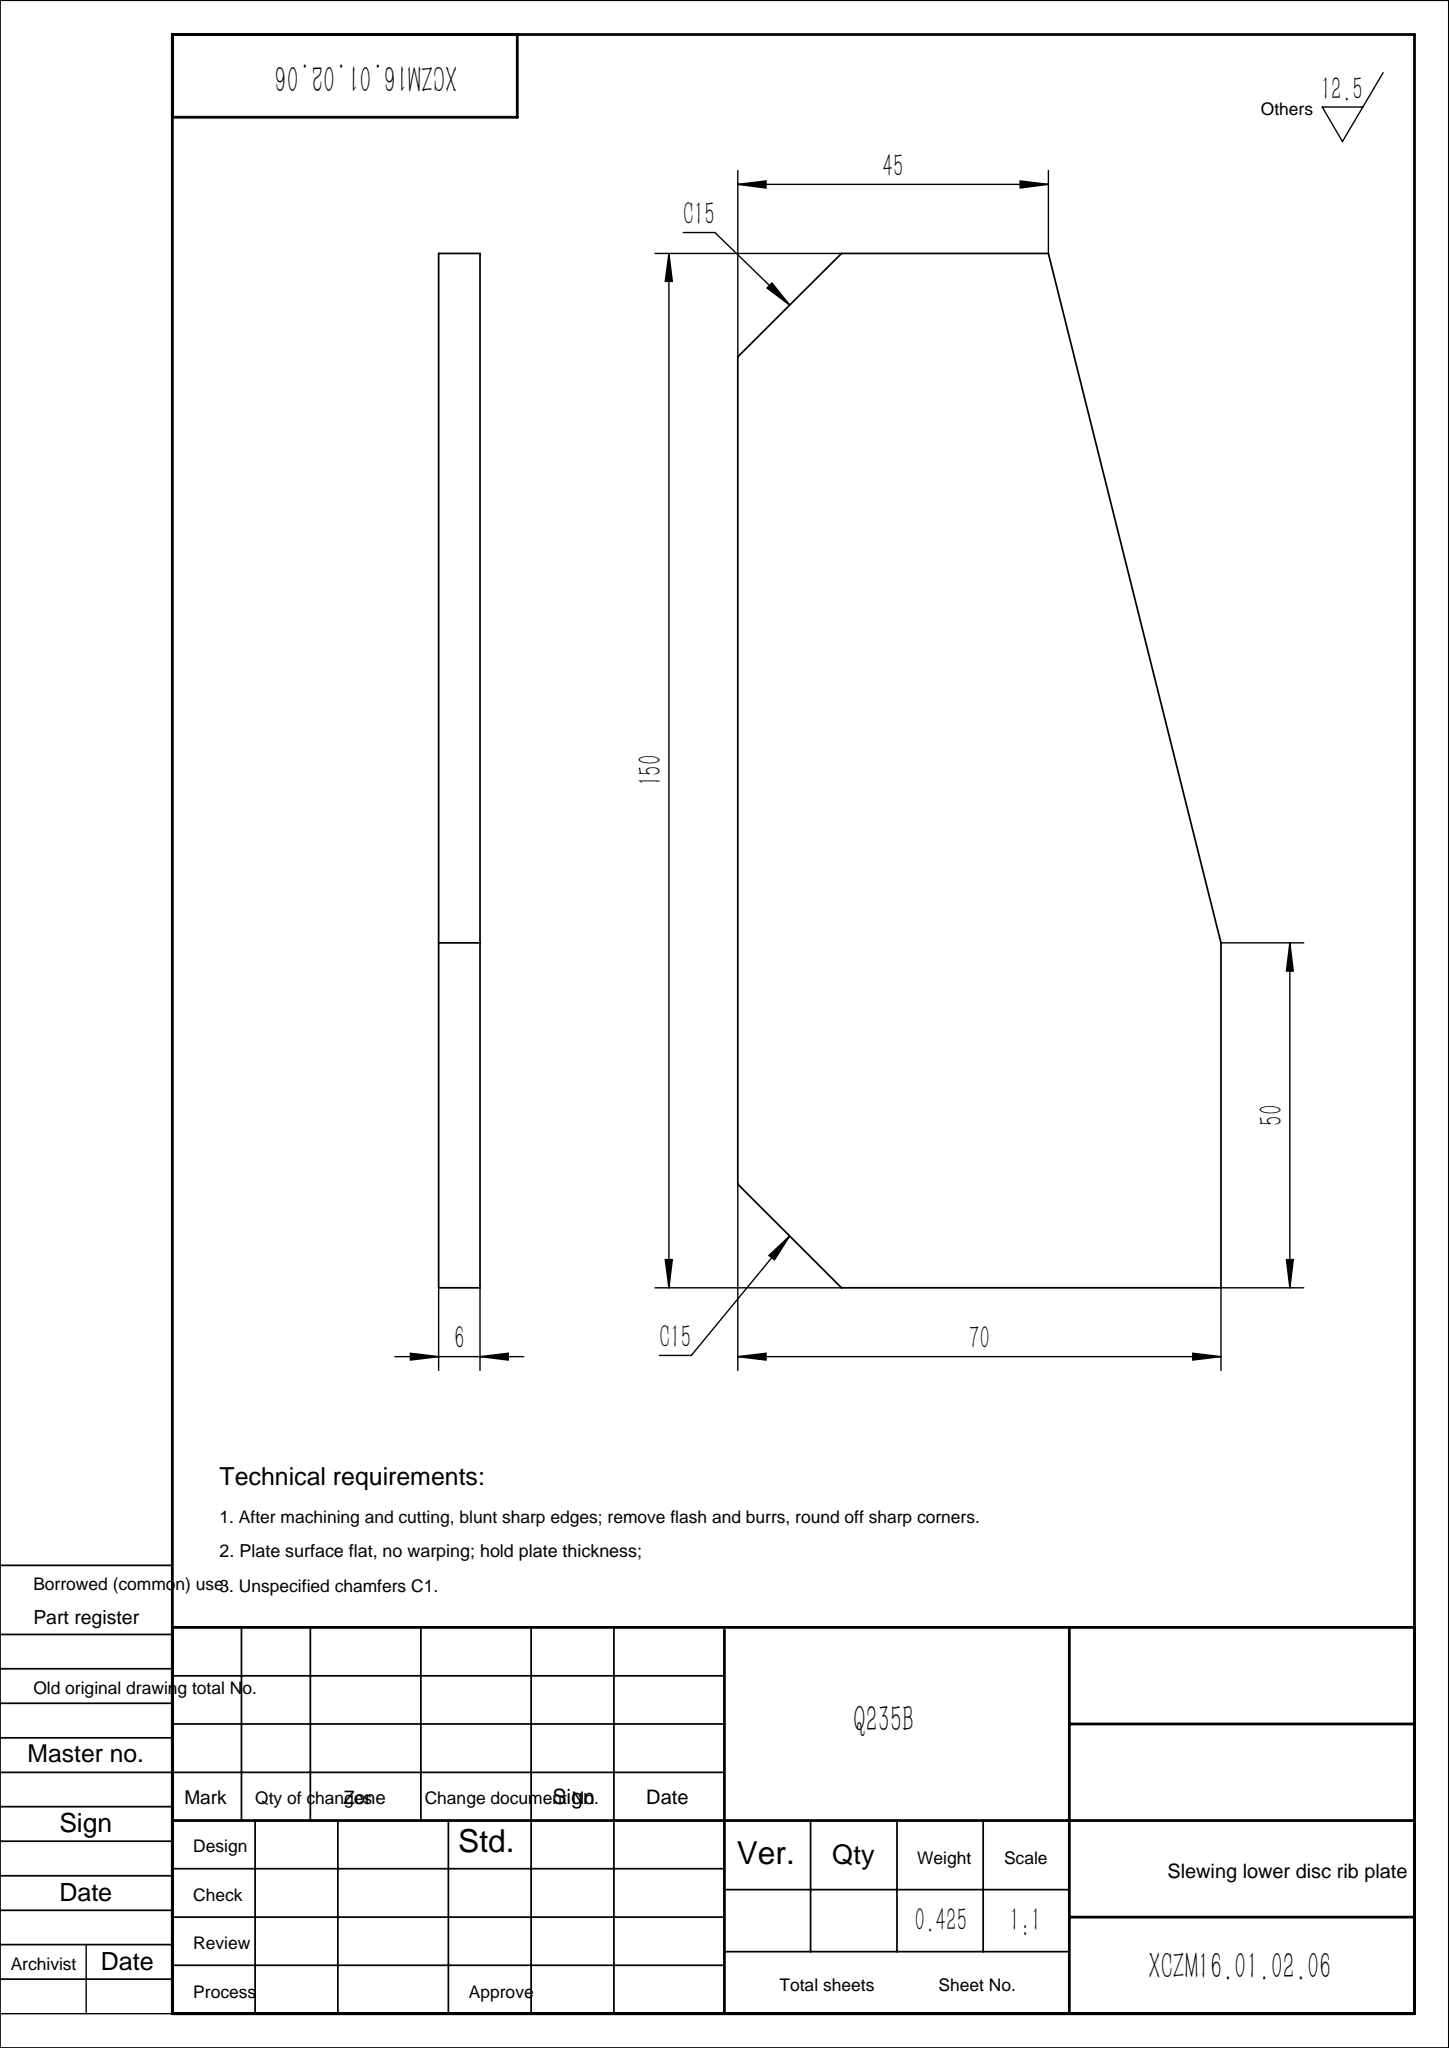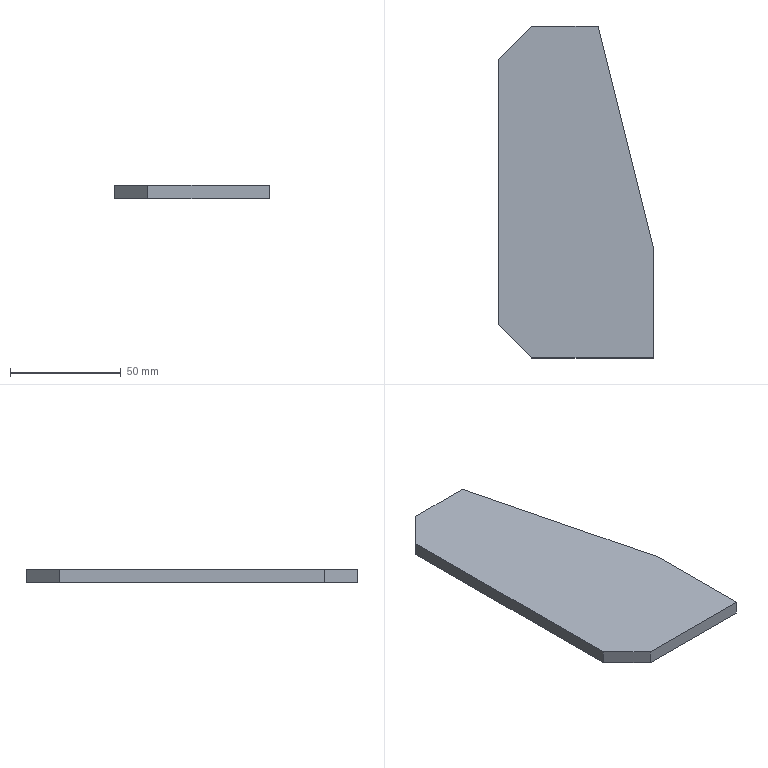Part | SolidWorks | features Chamfer 1, Extrusion 1 | 1 solid | 9 faces | box 70 x 150 x 6 mm | volume 54150 mm3 | plane 9
STEP:
#1=CARTESIAN_POINT('',(45.,150.,0.));
#2=VERTEX_POINT('',#1);
#3=CARTESIAN_POINT('',(15.,150.,0.));
#4=VERTEX_POINT('',#3);
#5=CARTESIAN_POINT('',(45.,150.,0.));
#6=DIRECTION('',(-1.,0.,0.));
#7=VECTOR('',#6,1000.);
#8=LINE('',#5,#7);
#9=EDGE_CURVE('',#2,#4,#8,.T.);
#10=ORIENTED_EDGE('',*,*,#9,.T.);
#11=CARTESIAN_POINT('',(15.,150.,6.));
#12=VERTEX_POINT('',#11);
#13=CARTESIAN_POINT('',(15.,150.,6.));
#14=DIRECTION('',(0.,0.,1.));
#15=VECTOR('',#14,1000.);
#16=LINE('',#13,#15);
#17=EDGE_CURVE('',#4,#12,#16,.T.);
#18=ORIENTED_EDGE('',*,*,#17,.T.);
#19=CARTESIAN_POINT('',(45.,150.,6.));
#20=VERTEX_POINT('',#19);
#21=CARTESIAN_POINT('',(45.,150.,6.));
#22=DIRECTION('',(-1.,0.,0.));
#23=VECTOR('',#22,1000.);
#24=LINE('',#21,#23);
#25=EDGE_CURVE('',#20,#12,#24,.T.);
#26=ORIENTED_EDGE('',*,*,#25,.F.);
#27=CARTESIAN_POINT('',(45.,150.,6.));
#28=DIRECTION('',(0.,0.,-1.));
#29=VECTOR('',#28,1000.);
#30=LINE('',#27,#29);
#31=EDGE_CURVE('',#20,#2,#30,.T.);
#32=ORIENTED_EDGE('',*,*,#31,.T.);
#33=EDGE_LOOP('',(#10,#18,#26,#32));
#34=FACE_OUTER_BOUND('',#33,.T.);
#35=CARTESIAN_POINT('',(45.,150.,6.));
#36=DIRECTION('',(0.,-1.,0.));
#37=DIRECTION('',(0.,0.,-1.));
#38=AXIS2_PLACEMENT_3D('',#35,#36,#37);
#39=PLANE('',#38);
#40=ADVANCED_FACE('',(#34),#39,.F.);
#41=CARTESIAN_POINT('',(0.,135.,6.));
#42=VERTEX_POINT('',#41);
#43=CARTESIAN_POINT('',(0.,15.,6.));
#44=VERTEX_POINT('',#43);
#45=CARTESIAN_POINT('',(0.,150.,6.));
#46=DIRECTION('',(0.,-1.,0.));
#47=VECTOR('',#46,1000.);
#48=LINE('',#45,#47);
#49=EDGE_CURVE('',#42,#44,#48,.T.);
#50=ORIENTED_EDGE('',*,*,#49,.F.);
#51=CARTESIAN_POINT('',(0.,135.,0.));
#52=VERTEX_POINT('',#51);
#53=CARTESIAN_POINT('',(0.,135.,6.));
#54=DIRECTION('',(0.,0.,-1.));
#55=VECTOR('',#54,1000.);
#56=LINE('',#53,#55);
#57=EDGE_CURVE('',#42,#52,#56,.T.);
#58=ORIENTED_EDGE('',*,*,#57,.T.);
#59=CARTESIAN_POINT('',(0.,15.,0.));
#60=VERTEX_POINT('',#59);
#61=CARTESIAN_POINT('',(0.,150.,0.));
#62=DIRECTION('',(0.,-1.,0.));
#63=VECTOR('',#62,1000.);
#64=LINE('',#61,#63);
#65=EDGE_CURVE('',#52,#60,#64,.T.);
#66=ORIENTED_EDGE('',*,*,#65,.T.);
#67=CARTESIAN_POINT('',(0.,15.,6.));
#68=DIRECTION('',(0.,0.,1.));
#69=VECTOR('',#68,1000.);
#70=LINE('',#67,#69);
#71=EDGE_CURVE('',#60,#44,#70,.T.);
#72=ORIENTED_EDGE('',*,*,#71,.T.);
#73=EDGE_LOOP('',(#50,#58,#66,#72));
#74=FACE_OUTER_BOUND('',#73,.T.);
#75=CARTESIAN_POINT('',(0.,150.,6.));
#76=DIRECTION('',(1.,0.,0.));
#77=DIRECTION('',(0.,1.,0.));
#78=AXIS2_PLACEMENT_3D('',#75,#76,#77);
#79=PLANE('',#78);
#80=ADVANCED_FACE('',(#74),#79,.F.);
#81=CARTESIAN_POINT('',(15.,0.,6.));
#82=VERTEX_POINT('',#81);
#83=CARTESIAN_POINT('',(70.,0.,6.));
#84=VERTEX_POINT('',#83);
#85=CARTESIAN_POINT('',(0.,0.,6.));
#86=DIRECTION('',(1.,0.,0.));
#87=VECTOR('',#86,1000.);
#88=LINE('',#85,#87);
#89=EDGE_CURVE('',#82,#84,#88,.T.);
#90=ORIENTED_EDGE('',*,*,#89,.F.);
#91=CARTESIAN_POINT('',(15.,0.,0.));
#92=VERTEX_POINT('',#91);
#93=CARTESIAN_POINT('',(15.,0.,6.));
#94=DIRECTION('',(0.,0.,-1.));
#95=VECTOR('',#94,1000.);
#96=LINE('',#93,#95);
#97=EDGE_CURVE('',#82,#92,#96,.T.);
#98=ORIENTED_EDGE('',*,*,#97,.T.);
#99=CARTESIAN_POINT('',(70.,0.,0.));
#100=VERTEX_POINT('',#99);
#101=CARTESIAN_POINT('',(0.,0.,0.));
#102=DIRECTION('',(1.,0.,0.));
#103=VECTOR('',#102,1000.);
#104=LINE('',#101,#103);
#105=EDGE_CURVE('',#92,#100,#104,.T.);
#106=ORIENTED_EDGE('',*,*,#105,.T.);
#107=CARTESIAN_POINT('',(70.,0.,6.));
#108=DIRECTION('',(0.,0.,-1.));
#109=VECTOR('',#108,1000.);
#110=LINE('',#107,#109);
#111=EDGE_CURVE('',#84,#100,#110,.T.);
#112=ORIENTED_EDGE('',*,*,#111,.F.);
#113=EDGE_LOOP('',(#90,#98,#106,#112));
#114=FACE_OUTER_BOUND('',#113,.T.);
#115=CARTESIAN_POINT('',(0.,0.,6.));
#116=DIRECTION('',(0.,1.,0.));
#117=DIRECTION('',(0.,0.,1.));
#118=AXIS2_PLACEMENT_3D('',#115,#116,#117);
#119=PLANE('',#118);
#120=ADVANCED_FACE('',(#114),#119,.F.);
#121=CARTESIAN_POINT('',(70.,50.,0.));
#122=VERTEX_POINT('',#121);
#123=CARTESIAN_POINT('',(70.,0.,0.));
#124=DIRECTION('',(0.,1.,0.));
#125=VECTOR('',#124,1000.);
#126=LINE('',#123,#125);
#127=EDGE_CURVE('',#100,#122,#126,.T.);
#128=ORIENTED_EDGE('',*,*,#127,.T.);
#129=CARTESIAN_POINT('',(70.,50.,6.));
#130=VERTEX_POINT('',#129);
#131=CARTESIAN_POINT('',(70.,50.,6.));
#132=DIRECTION('',(0.,0.,-1.));
#133=VECTOR('',#132,1000.);
#134=LINE('',#131,#133);
#135=EDGE_CURVE('',#130,#122,#134,.T.);
#136=ORIENTED_EDGE('',*,*,#135,.F.);
#137=CARTESIAN_POINT('',(70.,0.,6.));
#138=DIRECTION('',(0.,1.,0.));
#139=VECTOR('',#138,1000.);
#140=LINE('',#137,#139);
#141=EDGE_CURVE('',#84,#130,#140,.T.);
#142=ORIENTED_EDGE('',*,*,#141,.F.);
#143=ORIENTED_EDGE('',*,*,#111,.T.);
#144=EDGE_LOOP('',(#128,#136,#142,#143));
#145=FACE_OUTER_BOUND('',#144,.T.);
#146=CARTESIAN_POINT('',(70.,0.,6.));
#147=DIRECTION('',(-1.,0.,0.));
#148=DIRECTION('',(0.,0.,1.));
#149=AXIS2_PLACEMENT_3D('',#146,#147,#148);
#150=PLANE('',#149);
#151=ADVANCED_FACE('',(#145),#150,.F.);
#152=CARTESIAN_POINT('',(70.,50.,0.));
#153=DIRECTION('',(-0.2425,0.9701,0.));
#154=VECTOR('',#153,1000.);
#155=LINE('',#152,#154);
#156=EDGE_CURVE('',#122,#2,#155,.T.);
#157=ORIENTED_EDGE('',*,*,#156,.T.);
#158=ORIENTED_EDGE('',*,*,#31,.F.);
#159=CARTESIAN_POINT('',(70.,50.,6.));
#160=DIRECTION('',(-0.2425,0.9701,0.));
#161=VECTOR('',#160,1000.);
#162=LINE('',#159,#161);
#163=EDGE_CURVE('',#130,#20,#162,.T.);
#164=ORIENTED_EDGE('',*,*,#163,.F.);
#165=ORIENTED_EDGE('',*,*,#135,.T.);
#166=EDGE_LOOP('',(#157,#158,#164,#165));
#167=FACE_OUTER_BOUND('',#166,.T.);
#168=CARTESIAN_POINT('',(70.,50.,6.));
#169=DIRECTION('',(-0.9701,-0.2425,0.));
#170=DIRECTION('',(0.2425,-0.9701,0.));
#171=AXIS2_PLACEMENT_3D('',#168,#169,#170);
#172=PLANE('',#171);
#173=ADVANCED_FACE('',(#167),#172,.F.);
#174=ORIENTED_EDGE('',*,*,#25,.T.);
#175=CARTESIAN_POINT('',(-67.5,67.5,6.));
#176=DIRECTION('',(-0.7071,-0.7071,0.));
#177=VECTOR('',#176,1000.);
#178=LINE('',#175,#177);
#179=EDGE_CURVE('',#12,#42,#178,.T.);
#180=ORIENTED_EDGE('',*,*,#179,.T.);
#181=ORIENTED_EDGE('',*,*,#49,.T.);
#182=CARTESIAN_POINT('',(7.5,7.5,6.));
#183=DIRECTION('',(0.7071,-0.7071,0.));
#184=VECTOR('',#183,1000.);
#185=LINE('',#182,#184);
#186=EDGE_CURVE('',#44,#82,#185,.T.);
#187=ORIENTED_EDGE('',*,*,#186,.T.);
#188=ORIENTED_EDGE('',*,*,#89,.T.);
#189=ORIENTED_EDGE('',*,*,#141,.T.);
#190=ORIENTED_EDGE('',*,*,#163,.T.);
#191=EDGE_LOOP('',(#174,#180,#181,#187,#188,#189,#190));
#192=FACE_OUTER_BOUND('',#191,.T.);
#193=CARTESIAN_POINT('',(0.,0.,6.));
#194=DIRECTION('',(0.,0.,1.));
#195=DIRECTION('',(1.,0.,0.));
#196=AXIS2_PLACEMENT_3D('',#193,#194,#195);
#197=PLANE('',#196);
#198=ADVANCED_FACE('',(#192),#197,.T.);
#199=ORIENTED_EDGE('',*,*,#65,.F.);
#200=CARTESIAN_POINT('',(0.,135.,0.));
#201=DIRECTION('',(0.7071,0.7071,0.));
#202=VECTOR('',#201,1000.);
#203=LINE('',#200,#202);
#204=EDGE_CURVE('',#52,#4,#203,.T.);
#205=ORIENTED_EDGE('',*,*,#204,.T.);
#206=ORIENTED_EDGE('',*,*,#9,.F.);
#207=ORIENTED_EDGE('',*,*,#156,.F.);
#208=ORIENTED_EDGE('',*,*,#127,.F.);
#209=ORIENTED_EDGE('',*,*,#105,.F.);
#210=CARTESIAN_POINT('',(15.,0.,0.));
#211=DIRECTION('',(-0.7071,0.7071,0.));
#212=VECTOR('',#211,1000.);
#213=LINE('',#210,#212);
#214=EDGE_CURVE('',#92,#60,#213,.T.);
#215=ORIENTED_EDGE('',*,*,#214,.T.);
#216=EDGE_LOOP('',(#199,#205,#206,#207,#208,#209,#215));
#217=FACE_OUTER_BOUND('',#216,.T.);
#218=CARTESIAN_POINT('',(0.,0.,0.));
#219=DIRECTION('',(0.,0.,1.));
#220=DIRECTION('',(1.,0.,0.));
#221=AXIS2_PLACEMENT_3D('',#218,#219,#220);
#222=PLANE('',#221);
#223=ADVANCED_FACE('',(#217),#222,.F.);
#224=ORIENTED_EDGE('',*,*,#179,.F.);
#225=ORIENTED_EDGE('',*,*,#17,.F.);
#226=ORIENTED_EDGE('',*,*,#204,.F.);
#227=ORIENTED_EDGE('',*,*,#57,.F.);
#228=EDGE_LOOP('',(#224,#225,#226,#227));
#229=FACE_OUTER_BOUND('',#228,.T.);
#230=CARTESIAN_POINT('',(0.,135.,6.));
#231=DIRECTION('',(0.7071,-0.7071,0.));
#232=DIRECTION('',(0.,0.,-1.));
#233=AXIS2_PLACEMENT_3D('',#230,#231,#232);
#234=PLANE('',#233);
#235=ADVANCED_FACE('',(#229),#234,.F.);
#236=ORIENTED_EDGE('',*,*,#186,.F.);
#237=ORIENTED_EDGE('',*,*,#71,.F.);
#238=ORIENTED_EDGE('',*,*,#214,.F.);
#239=ORIENTED_EDGE('',*,*,#97,.F.);
#240=EDGE_LOOP('',(#236,#237,#238,#239));
#241=FACE_OUTER_BOUND('',#240,.T.);
#242=CARTESIAN_POINT('',(15.,0.,6.));
#243=DIRECTION('',(0.7071,0.7071,0.));
#244=DIRECTION('',(0.,0.,-1.));
#245=AXIS2_PLACEMENT_3D('',#242,#243,#244);
#246=PLANE('',#245);
#247=ADVANCED_FACE('',(#241),#246,.F.);
#248=CLOSED_SHELL('',(#40,#80,#120,#151,#173,#198,#223,#235,#247));
#249=MANIFOLD_SOLID_BREP('',#248);
#250=CARTESIAN_POINT('',(0.,0.,0.));
#251=DIRECTION('',(0.,0.,1.));
#252=DIRECTION('',(1.,0.,0.));
#253=AXIS2_PLACEMENT_3D('',#250,#251,#252);
#254=(LENGTH_UNIT()NAMED_UNIT(*)SI_UNIT(.MILLI.,.METRE.));
#255=UNCERTAINTY_MEASURE_WITH_UNIT(LENGTH_MEASURE(0.00001),#254,'','');
#256=(NAMED_UNIT(*)PLANE_ANGLE_UNIT()SI_UNIT($,.RADIAN.));
#257=(NAMED_UNIT(*)SI_UNIT($,.STERADIAN.)SOLID_ANGLE_UNIT());
#258=(GEOMETRIC_REPRESENTATION_CONTEXT(3)GLOBAL_UNCERTAINTY_ASSIGNED_CONTEXT((#255))GLOBAL_UNIT_ASSIGNED_CONTEXT((#254,#256,#257))REPRESENTATION_CONTEXT('',''));
#259=ADVANCED_BREP_SHAPE_REPRESENTATION('',(#249,#253),#258);